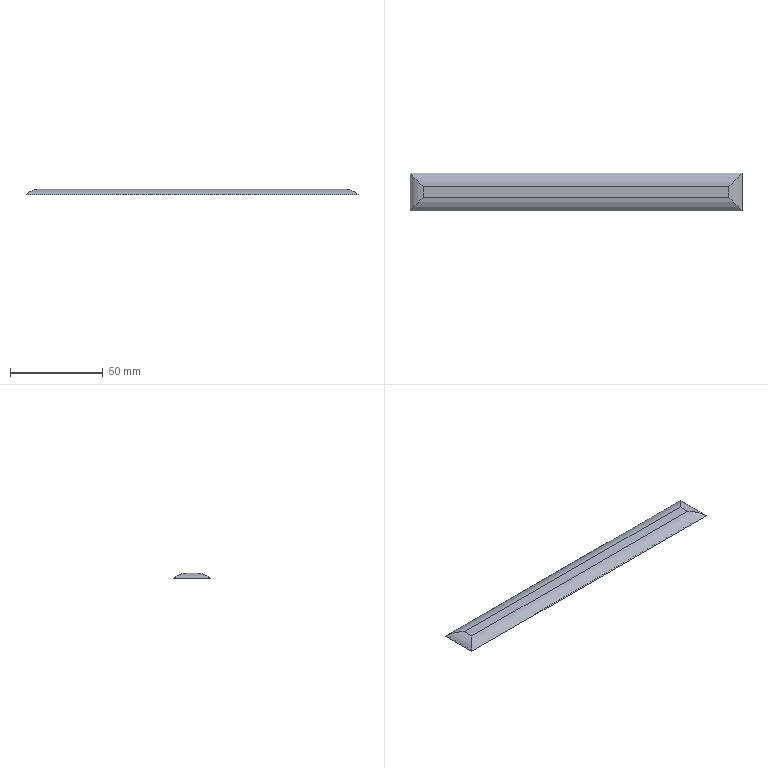Part | SolidWorks | features Extrusion 1, Fillet 1, Shell 1 | 1 solid | 11 faces | box 178.57 x 20 x 3 mm | volume 1853 mm3 | cylinder 8 | plane 3 | commonest cylinder face diameters 19 x4 20 x4
STEP:
#1=CARTESIAN_POINT('',(89.285,-10.,0.));
#2=VERTEX_POINT('',#1);
#3=CARTESIAN_POINT('',(89.285,10.,0.));
#4=VERTEX_POINT('',#3);
#5=CARTESIAN_POINT('',(89.285,-10.,0.));
#6=DIRECTION('',(0.,1.,0.));
#7=VECTOR('',#6,1000.);
#8=LINE('',#5,#7);
#9=EDGE_CURVE('',#2,#4,#8,.T.);
#10=ORIENTED_EDGE('',*,*,#9,.F.);
#11=CARTESIAN_POINT('',(-89.285,-10.,0.));
#12=VERTEX_POINT('',#11);
#13=CARTESIAN_POINT('',(-89.285,-10.,0.));
#14=DIRECTION('',(1.,0.,0.));
#15=VECTOR('',#14,1000.);
#16=LINE('',#13,#15);
#17=EDGE_CURVE('',#12,#2,#16,.T.);
#18=ORIENTED_EDGE('',*,*,#17,.F.);
#19=CARTESIAN_POINT('',(-89.285,10.,0.));
#20=VERTEX_POINT('',#19);
#21=CARTESIAN_POINT('',(-89.285,-10.,0.));
#22=DIRECTION('',(0.,-1.,0.));
#23=VECTOR('',#22,1000.);
#24=LINE('',#21,#23);
#25=EDGE_CURVE('',#20,#12,#24,.T.);
#26=ORIENTED_EDGE('',*,*,#25,.F.);
#27=CARTESIAN_POINT('',(-89.285,10.,0.));
#28=DIRECTION('',(-1.,0.,0.));
#29=VECTOR('',#28,1000.);
#30=LINE('',#27,#29);
#31=EDGE_CURVE('',#4,#20,#30,.T.);
#32=ORIENTED_EDGE('',*,*,#31,.F.);
#33=EDGE_LOOP('',(#10,#18,#26,#32));
#34=FACE_OUTER_BOUND('',#33,.T.);
#35=CARTESIAN_POINT('',(-88.566,-9.281,0.));
#36=VERTEX_POINT('',#35);
#37=CARTESIAN_POINT('',(88.566,-9.281,0.));
#38=VERTEX_POINT('',#37);
#39=CARTESIAN_POINT('',(-88.566,-9.281,0.));
#40=DIRECTION('',(1.,0.,0.));
#41=VECTOR('',#40,1000.);
#42=LINE('',#39,#41);
#43=EDGE_CURVE('',#36,#38,#42,.T.);
#44=ORIENTED_EDGE('',*,*,#43,.T.);
#45=CARTESIAN_POINT('',(88.566,9.281,0.));
#46=VERTEX_POINT('',#45);
#47=CARTESIAN_POINT('',(88.566,-9.281,0.));
#48=DIRECTION('',(0.,1.,0.));
#49=VECTOR('',#48,1000.);
#50=LINE('',#47,#49);
#51=EDGE_CURVE('',#38,#46,#50,.T.);
#52=ORIENTED_EDGE('',*,*,#51,.T.);
#53=CARTESIAN_POINT('',(-88.566,9.281,0.));
#54=VERTEX_POINT('',#53);
#55=CARTESIAN_POINT('',(88.566,9.281,0.));
#56=DIRECTION('',(-1.,0.,0.));
#57=VECTOR('',#56,1000.);
#58=LINE('',#55,#57);
#59=EDGE_CURVE('',#46,#54,#58,.T.);
#60=ORIENTED_EDGE('',*,*,#59,.T.);
#61=CARTESIAN_POINT('',(-88.566,9.281,0.));
#62=DIRECTION('',(0.,-1.,0.));
#63=VECTOR('',#62,1000.);
#64=LINE('',#61,#63);
#65=EDGE_CURVE('',#54,#36,#64,.T.);
#66=ORIENTED_EDGE('',*,*,#65,.T.);
#67=EDGE_LOOP('',(#44,#52,#60,#66));
#68=FACE_BOUND('',#67,.T.);
#69=CARTESIAN_POINT('',(0.,0.,0.));
#70=DIRECTION('',(0.,0.,-1.));
#71=DIRECTION('',(-1.,0.,0.));
#72=AXIS2_PLACEMENT_3D('',#69,#70,#71);
#73=PLANE('',#72);
#74=ADVANCED_FACE('',(#34,#68),#73,.T.);
#75=CARTESIAN_POINT('',(-82.144,2.859,3.));
#76=VERTEX_POINT('',#75);
#77=CARTESIAN_POINT('',(-82.144,-2.859,3.));
#78=VERTEX_POINT('',#77);
#79=CARTESIAN_POINT('',(-82.144,0.,3.));
#80=DIRECTION('',(0.,-1.,0.));
#81=VECTOR('',#80,1000.);
#82=LINE('',#79,#81);
#83=EDGE_CURVE('',#76,#78,#82,.T.);
#84=ORIENTED_EDGE('',*,*,#83,.T.);
#85=CARTESIAN_POINT('',(82.144,-2.859,3.));
#86=VERTEX_POINT('',#85);
#87=CARTESIAN_POINT('',(0.,-2.859,3.));
#88=DIRECTION('',(1.,0.,0.));
#89=VECTOR('',#88,1000.);
#90=LINE('',#87,#89);
#91=EDGE_CURVE('',#78,#86,#90,.T.);
#92=ORIENTED_EDGE('',*,*,#91,.T.);
#93=CARTESIAN_POINT('',(82.144,2.859,3.));
#94=VERTEX_POINT('',#93);
#95=CARTESIAN_POINT('',(82.144,0.,3.));
#96=DIRECTION('',(0.,1.,0.));
#97=VECTOR('',#96,1000.);
#98=LINE('',#95,#97);
#99=EDGE_CURVE('',#86,#94,#98,.T.);
#100=ORIENTED_EDGE('',*,*,#99,.T.);
#101=CARTESIAN_POINT('',(0.,2.859,3.));
#102=DIRECTION('',(-1.,0.,0.));
#103=VECTOR('',#102,1000.);
#104=LINE('',#101,#103);
#105=EDGE_CURVE('',#94,#76,#104,.T.);
#106=ORIENTED_EDGE('',*,*,#105,.T.);
#107=EDGE_LOOP('',(#84,#92,#100,#106));
#108=FACE_OUTER_BOUND('',#107,.T.);
#109=CARTESIAN_POINT('',(0.,0.,3.));
#110=DIRECTION('',(0.,0.,-1.));
#111=DIRECTION('',(-1.,0.,0.));
#112=AXIS2_PLACEMENT_3D('',#109,#110,#111);
#113=PLANE('',#112);
#114=ADVANCED_FACE('',(#108),#113,.F.);
#115=CARTESIAN_POINT('',(89.285,10.,0.));
#116=CARTESIAN_POINT('',(87.378,8.093,1.945));
#117=CARTESIAN_POINT('',(84.867,5.582,3.));
#118=CARTESIAN_POINT('',(82.144,2.859,3.));
#119=(BOUNDED_CURVE()B_SPLINE_CURVE(3,(#115,#116,#117,#118),.UNSPECIFIED.,.F.,.F.)B_SPLINE_CURVE_WITH_KNOTS((4,4),(3.917,4.712),.UNSPECIFIED.)CURVE()GEOMETRIC_REPRESENTATION_ITEM()RATIONAL_B_SPLINE_CURVE((1.,0.948,0.948,1.))REPRESENTATION_ITEM(''));
#120=EDGE_CURVE('',#4,#94,#119,.T.);
#121=ORIENTED_EDGE('',*,*,#120,.F.);
#122=ORIENTED_EDGE('',*,*,#31,.T.);
#123=CARTESIAN_POINT('',(-82.144,2.859,3.));
#124=CARTESIAN_POINT('',(-84.867,5.582,3.));
#125=CARTESIAN_POINT('',(-87.378,8.093,1.945));
#126=CARTESIAN_POINT('',(-89.285,10.,0.));
#127=(BOUNDED_CURVE()B_SPLINE_CURVE(3,(#123,#124,#125,#126),.UNSPECIFIED.,.F.,.F.)B_SPLINE_CURVE_WITH_KNOTS((4,4),(1.571,2.366),.UNSPECIFIED.)CURVE()GEOMETRIC_REPRESENTATION_ITEM()RATIONAL_B_SPLINE_CURVE((1.,0.948,0.948,1.))REPRESENTATION_ITEM(''));
#128=EDGE_CURVE('',#76,#20,#127,.T.);
#129=ORIENTED_EDGE('',*,*,#128,.F.);
#130=ORIENTED_EDGE('',*,*,#105,.F.);
#131=EDGE_LOOP('',(#121,#122,#129,#130));
#132=FACE_OUTER_BOUND('',#131,.T.);
#133=CARTESIAN_POINT('',(-89.285,2.859,-7.));
#134=DIRECTION('',(1.,0.,0.));
#135=DIRECTION('',(0.,0.,-1.));
#136=AXIS2_PLACEMENT_3D('',#133,#134,#135);
#137=CYLINDRICAL_SURFACE('',#136,10.);
#138=ADVANCED_FACE('',(#132),#137,.T.);
#139=ORIENTED_EDGE('',*,*,#128,.T.);
#140=ORIENTED_EDGE('',*,*,#25,.T.);
#141=CARTESIAN_POINT('',(-82.144,-2.859,3.));
#142=CARTESIAN_POINT('',(-84.867,-5.582,3.));
#143=CARTESIAN_POINT('',(-87.378,-8.093,1.945));
#144=CARTESIAN_POINT('',(-89.285,-10.,0.));
#145=(BOUNDED_CURVE()B_SPLINE_CURVE(3,(#141,#142,#143,#144),.UNSPECIFIED.,.F.,.F.)B_SPLINE_CURVE_WITH_KNOTS((4,4),(1.571,2.366),.UNSPECIFIED.)CURVE()GEOMETRIC_REPRESENTATION_ITEM()RATIONAL_B_SPLINE_CURVE((1.,0.948,0.948,1.))REPRESENTATION_ITEM(''));
#146=EDGE_CURVE('',#78,#12,#145,.T.);
#147=ORIENTED_EDGE('',*,*,#146,.F.);
#148=ORIENTED_EDGE('',*,*,#83,.F.);
#149=EDGE_LOOP('',(#139,#140,#147,#148));
#150=FACE_OUTER_BOUND('',#149,.T.);
#151=CARTESIAN_POINT('',(-82.144,-10.,-7.));
#152=DIRECTION('',(0.,1.,0.));
#153=DIRECTION('',(0.,0.,1.));
#154=AXIS2_PLACEMENT_3D('',#151,#152,#153);
#155=CYLINDRICAL_SURFACE('',#154,10.);
#156=ADVANCED_FACE('',(#150),#155,.T.);
#157=ORIENTED_EDGE('',*,*,#120,.T.);
#158=ORIENTED_EDGE('',*,*,#99,.F.);
#159=CARTESIAN_POINT('',(89.285,-10.,0.));
#160=CARTESIAN_POINT('',(87.378,-8.093,1.945));
#161=CARTESIAN_POINT('',(84.867,-5.582,3.));
#162=CARTESIAN_POINT('',(82.144,-2.859,3.));
#163=(BOUNDED_CURVE()B_SPLINE_CURVE(3,(#159,#160,#161,#162),.UNSPECIFIED.,.F.,.F.)B_SPLINE_CURVE_WITH_KNOTS((4,4),(0.7754,1.571),.UNSPECIFIED.)CURVE()GEOMETRIC_REPRESENTATION_ITEM()RATIONAL_B_SPLINE_CURVE((1.,0.948,0.948,1.))REPRESENTATION_ITEM(''));
#164=EDGE_CURVE('',#2,#86,#163,.T.);
#165=ORIENTED_EDGE('',*,*,#164,.F.);
#166=ORIENTED_EDGE('',*,*,#9,.T.);
#167=EDGE_LOOP('',(#157,#158,#165,#166));
#168=FACE_OUTER_BOUND('',#167,.T.);
#169=CARTESIAN_POINT('',(82.144,-10.,-7.));
#170=DIRECTION('',(0.,-1.,0.));
#171=DIRECTION('',(0.,0.,-1.));
#172=AXIS2_PLACEMENT_3D('',#169,#170,#171);
#173=CYLINDRICAL_SURFACE('',#172,10.);
#174=ADVANCED_FACE('',(#168),#173,.T.);
#175=ORIENTED_EDGE('',*,*,#146,.T.);
#176=ORIENTED_EDGE('',*,*,#17,.T.);
#177=ORIENTED_EDGE('',*,*,#164,.T.);
#178=ORIENTED_EDGE('',*,*,#91,.F.);
#179=EDGE_LOOP('',(#175,#176,#177,#178));
#180=FACE_OUTER_BOUND('',#179,.T.);
#181=CARTESIAN_POINT('',(-89.285,-2.859,-7.));
#182=DIRECTION('',(-1.,0.,0.));
#183=DIRECTION('',(0.,0.,1.));
#184=AXIS2_PLACEMENT_3D('',#181,#182,#183);
#185=CYLINDRICAL_SURFACE('',#184,10.);
#186=ADVANCED_FACE('',(#180),#185,.T.);
#187=CARTESIAN_POINT('',(-82.144,2.859,2.5));
#188=VERTEX_POINT('',#187);
#189=CARTESIAN_POINT('',(-82.144,-2.859,2.5));
#190=VERTEX_POINT('',#189);
#191=CARTESIAN_POINT('',(-82.144,0.,2.5));
#192=DIRECTION('',(0.,-1.,0.));
#193=VECTOR('',#192,1000.);
#194=LINE('',#191,#193);
#195=EDGE_CURVE('',#188,#190,#194,.T.);
#196=ORIENTED_EDGE('',*,*,#195,.F.);
#197=CARTESIAN_POINT('',(82.144,2.859,2.5));
#198=VERTEX_POINT('',#197);
#199=CARTESIAN_POINT('',(0.,2.859,2.5));
#200=DIRECTION('',(-1.,0.,0.));
#201=VECTOR('',#200,1000.);
#202=LINE('',#199,#201);
#203=EDGE_CURVE('',#198,#188,#202,.T.);
#204=ORIENTED_EDGE('',*,*,#203,.F.);
#205=CARTESIAN_POINT('',(82.144,-2.859,2.5));
#206=VERTEX_POINT('',#205);
#207=CARTESIAN_POINT('',(82.144,0.,2.5));
#208=DIRECTION('',(0.,1.,0.));
#209=VECTOR('',#208,1000.);
#210=LINE('',#207,#209);
#211=EDGE_CURVE('',#206,#198,#210,.T.);
#212=ORIENTED_EDGE('',*,*,#211,.F.);
#213=CARTESIAN_POINT('',(0.,-2.859,2.5));
#214=DIRECTION('',(1.,0.,0.));
#215=VECTOR('',#214,1000.);
#216=LINE('',#213,#215);
#217=EDGE_CURVE('',#190,#206,#216,.T.);
#218=ORIENTED_EDGE('',*,*,#217,.F.);
#219=EDGE_LOOP('',(#196,#204,#212,#218));
#220=FACE_OUTER_BOUND('',#219,.T.);
#221=CARTESIAN_POINT('',(0.,0.,2.5));
#222=DIRECTION('',(0.,0.,-1.));
#223=DIRECTION('',(-1.,0.,0.));
#224=AXIS2_PLACEMENT_3D('',#221,#222,#223);
#225=PLANE('',#224);
#226=ADVANCED_FACE('',(#220),#225,.T.);
#227=CARTESIAN_POINT('',(88.566,9.281,0.));
#228=CARTESIAN_POINT('',(86.793,7.508,1.627));
#229=CARTESIAN_POINT('',(84.55,5.265,2.5));
#230=CARTESIAN_POINT('',(82.144,2.859,2.5));
#231=(BOUNDED_CURVE()B_SPLINE_CURVE(3,(#227,#228,#229,#230),.UNSPECIFIED.,.F.,.F.)B_SPLINE_CURVE_WITH_KNOTS((4,4),(3.97,4.712),.UNSPECIFIED.)CURVE()GEOMETRIC_REPRESENTATION_ITEM()RATIONAL_B_SPLINE_CURVE((1.,0.9546,0.9546,1.))REPRESENTATION_ITEM(''));
#232=EDGE_CURVE('',#46,#198,#231,.T.);
#233=ORIENTED_EDGE('',*,*,#232,.T.);
#234=ORIENTED_EDGE('',*,*,#203,.T.);
#235=CARTESIAN_POINT('',(-82.144,2.859,2.5));
#236=CARTESIAN_POINT('',(-84.55,5.265,2.5));
#237=CARTESIAN_POINT('',(-86.793,7.508,1.627));
#238=CARTESIAN_POINT('',(-88.566,9.281,0.));
#239=(BOUNDED_CURVE()B_SPLINE_CURVE(3,(#235,#236,#237,#238),.UNSPECIFIED.,.F.,.F.)B_SPLINE_CURVE_WITH_KNOTS((4,4),(4.712,5.455),.UNSPECIFIED.)CURVE()GEOMETRIC_REPRESENTATION_ITEM()RATIONAL_B_SPLINE_CURVE((1.,0.9546,0.9546,1.))REPRESENTATION_ITEM(''));
#240=EDGE_CURVE('',#188,#54,#239,.T.);
#241=ORIENTED_EDGE('',*,*,#240,.T.);
#242=ORIENTED_EDGE('',*,*,#59,.F.);
#243=EDGE_LOOP('',(#233,#234,#241,#242));
#244=FACE_OUTER_BOUND('',#243,.T.);
#245=CARTESIAN_POINT('',(-89.285,2.859,-7.));
#246=DIRECTION('',(1.,0.,0.));
#247=DIRECTION('',(0.,0.,-1.));
#248=AXIS2_PLACEMENT_3D('',#245,#246,#247);
#249=CYLINDRICAL_SURFACE('',#248,9.5);
#250=ADVANCED_FACE('',(#244),#249,.F.);
#251=ORIENTED_EDGE('',*,*,#240,.F.);
#252=ORIENTED_EDGE('',*,*,#195,.T.);
#253=CARTESIAN_POINT('',(-82.144,-2.859,2.5));
#254=CARTESIAN_POINT('',(-84.55,-5.265,2.5));
#255=CARTESIAN_POINT('',(-86.793,-7.508,1.627));
#256=CARTESIAN_POINT('',(-88.566,-9.281,0.));
#257=(BOUNDED_CURVE()B_SPLINE_CURVE(3,(#253,#254,#255,#256),.UNSPECIFIED.,.F.,.F.)B_SPLINE_CURVE_WITH_KNOTS((4,4),(4.712,5.455),.UNSPECIFIED.)CURVE()GEOMETRIC_REPRESENTATION_ITEM()RATIONAL_B_SPLINE_CURVE((1.,0.9546,0.9546,1.))REPRESENTATION_ITEM(''));
#258=EDGE_CURVE('',#190,#36,#257,.T.);
#259=ORIENTED_EDGE('',*,*,#258,.T.);
#260=ORIENTED_EDGE('',*,*,#65,.F.);
#261=EDGE_LOOP('',(#251,#252,#259,#260));
#262=FACE_OUTER_BOUND('',#261,.T.);
#263=CARTESIAN_POINT('',(-82.144,-10.,-7.));
#264=DIRECTION('',(0.,1.,0.));
#265=DIRECTION('',(0.,0.,1.));
#266=AXIS2_PLACEMENT_3D('',#263,#264,#265);
#267=CYLINDRICAL_SURFACE('',#266,9.5);
#268=ADVANCED_FACE('',(#262),#267,.F.);
#269=ORIENTED_EDGE('',*,*,#232,.F.);
#270=ORIENTED_EDGE('',*,*,#51,.F.);
#271=CARTESIAN_POINT('',(88.566,-9.281,0.));
#272=CARTESIAN_POINT('',(86.793,-7.508,1.627));
#273=CARTESIAN_POINT('',(84.55,-5.265,2.5));
#274=CARTESIAN_POINT('',(82.144,-2.859,2.5));
#275=(BOUNDED_CURVE()B_SPLINE_CURVE(3,(#271,#272,#273,#274),.UNSPECIFIED.,.F.,.F.)B_SPLINE_CURVE_WITH_KNOTS((4,4),(3.97,4.712),.UNSPECIFIED.)CURVE()GEOMETRIC_REPRESENTATION_ITEM()RATIONAL_B_SPLINE_CURVE((1.,0.9546,0.9546,1.))REPRESENTATION_ITEM(''));
#276=EDGE_CURVE('',#38,#206,#275,.T.);
#277=ORIENTED_EDGE('',*,*,#276,.T.);
#278=ORIENTED_EDGE('',*,*,#211,.T.);
#279=EDGE_LOOP('',(#269,#270,#277,#278));
#280=FACE_OUTER_BOUND('',#279,.T.);
#281=CARTESIAN_POINT('',(82.144,-10.,-7.));
#282=DIRECTION('',(0.,-1.,0.));
#283=DIRECTION('',(0.,0.,-1.));
#284=AXIS2_PLACEMENT_3D('',#281,#282,#283);
#285=CYLINDRICAL_SURFACE('',#284,9.5);
#286=ADVANCED_FACE('',(#280),#285,.F.);
#287=ORIENTED_EDGE('',*,*,#258,.F.);
#288=ORIENTED_EDGE('',*,*,#217,.T.);
#289=ORIENTED_EDGE('',*,*,#276,.F.);
#290=ORIENTED_EDGE('',*,*,#43,.F.);
#291=EDGE_LOOP('',(#287,#288,#289,#290));
#292=FACE_OUTER_BOUND('',#291,.T.);
#293=CARTESIAN_POINT('',(-89.285,-2.859,-7.));
#294=DIRECTION('',(-1.,0.,0.));
#295=DIRECTION('',(0.,0.,1.));
#296=AXIS2_PLACEMENT_3D('',#293,#294,#295);
#297=CYLINDRICAL_SURFACE('',#296,9.5);
#298=ADVANCED_FACE('',(#292),#297,.F.);
#299=CLOSED_SHELL('',(#74,#114,#138,#156,#174,#186,#226,#250,#268,#286,#298));
#300=MANIFOLD_SOLID_BREP('',#299);
#301=CARTESIAN_POINT('',(0.,0.,0.));
#302=DIRECTION('',(0.,0.,1.));
#303=DIRECTION('',(1.,0.,0.));
#304=AXIS2_PLACEMENT_3D('',#301,#302,#303);
#305=(LENGTH_UNIT()NAMED_UNIT(*)SI_UNIT(.MILLI.,.METRE.));
#306=UNCERTAINTY_MEASURE_WITH_UNIT(LENGTH_MEASURE(0.00001),#305,'','');
#307=(NAMED_UNIT(*)PLANE_ANGLE_UNIT()SI_UNIT($,.RADIAN.));
#308=(NAMED_UNIT(*)SI_UNIT($,.STERADIAN.)SOLID_ANGLE_UNIT());
#309=(GEOMETRIC_REPRESENTATION_CONTEXT(3)GLOBAL_UNCERTAINTY_ASSIGNED_CONTEXT((#306))GLOBAL_UNIT_ASSIGNED_CONTEXT((#305,#307,#308))REPRESENTATION_CONTEXT('',''));
#310=ADVANCED_BREP_SHAPE_REPRESENTATION('',(#300,#304),#309);